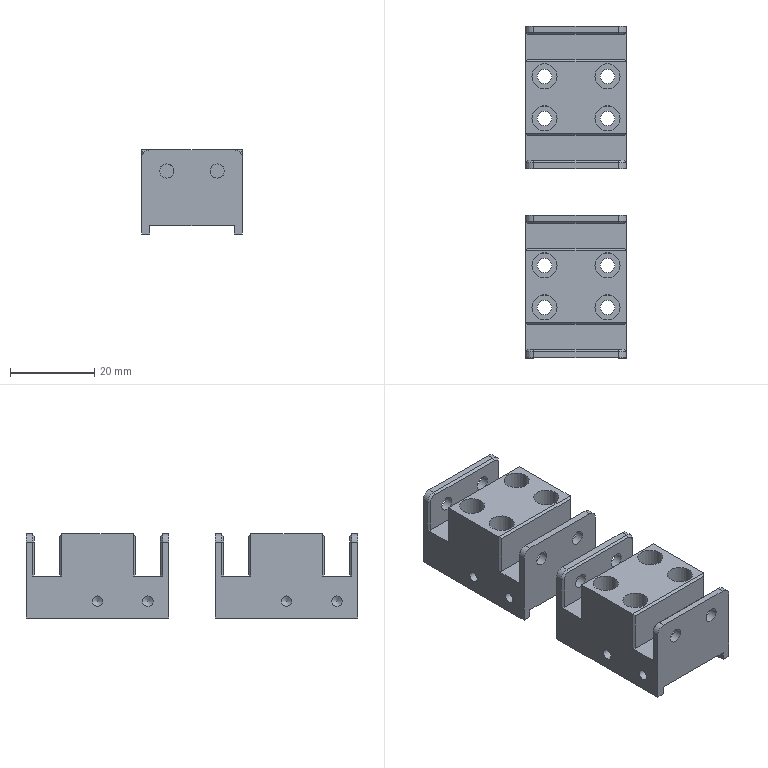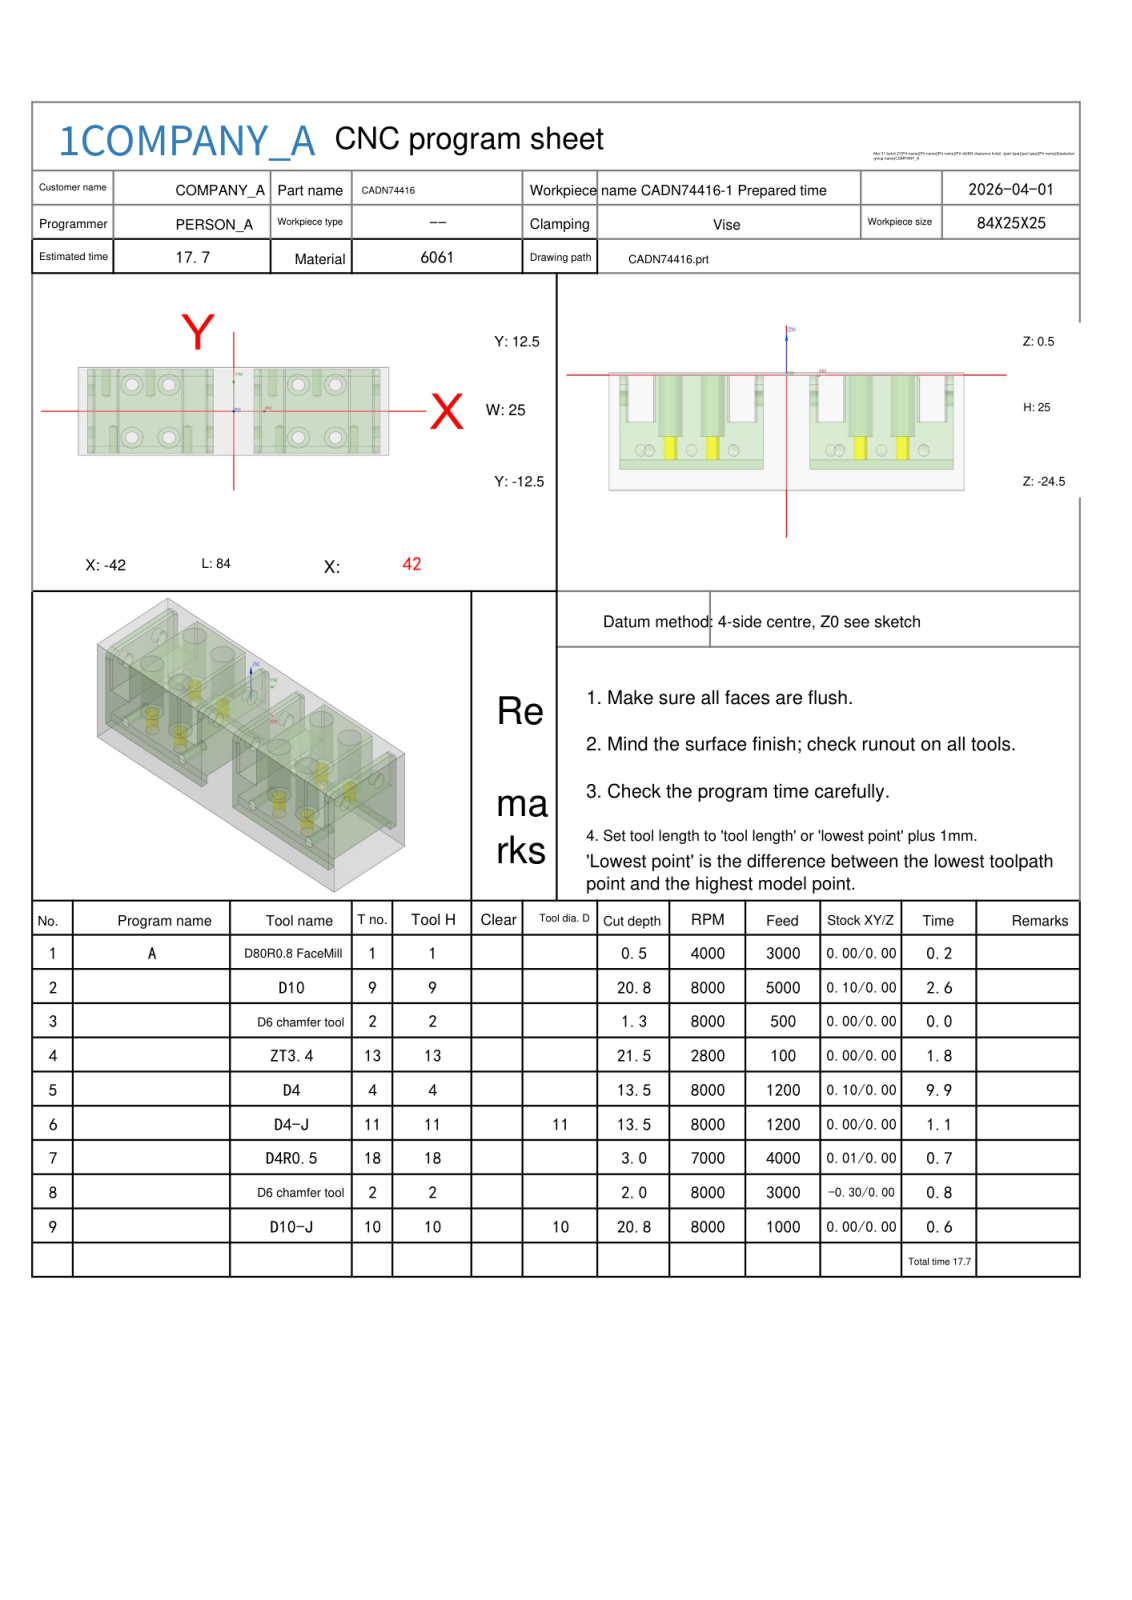NC program | NX | posted by the shop | part box 24 x 79 x 20 mm
Lines 4217 to 5292 of 7697:
N7 T18 M06
(D4R0.5  D=4. R=0.5 H=18 ce=0.01 di=0.00)
G00 G90 G54 X35.996 Y8.516 M03 S7000
G43 H18 Z10.5
M08
Z.491
G01 Z-.009 F4000.
X36.009 Y8.515
X36.024
G03 X36.424 Y8.9 I0.0 J.4
G01 X36.486 Y10.574
G02 X38. Y11.721 I1.656 J-.613
G01 X39.5
G03 X40.317 Y11.595 I.817 J2.584
X40.601 Y11.61 I0.0 J2.71
G01 Y11.646 Z-.014
Y11.681 Z-.018
G02 X39.5 Y11.812 I.04 J5.024
G01 X38.
G03 X36.378 Y10.29 I.095 J-1.726
G01 X36.373 Y10.255
X36.36 Y8.9
X36.326 Z-.03
X36.347 Y10.202
G02 X38. Y11.894 I1.721 J-.028
G01 X39.5
G03 X40.598 Y11.747 I1.098 J4.039
G01 X40.6
Y11.8 Z-.037
Y11.819 Z-.044
X39.5 Y11.976
X38.
G03 X36.315 Y10.23 I.098 J-1.781
G01 X36.288 Y8.9
X36.254 Z-.06
X36.278 Y10.29
X36.324 Y10.574
G02 X38. Y12.056 I1.748 J-.288
G01 X39.5
G02 X40.6 Y11.903 I-6.094 J-47.836
G01 Y11.957 Z-.07
Y11.997 Z-.08
G02 X39.5 Y12.136 I.262 J6.5
G01 X38.
G03 X36.302 Y10.663 I.069 J-1.795
G01 X36.234 Y10.29
X36.222 Y8.9
X36.188 Z-.102
X36.207 Y10.29
G02 X37.223 Y12.018 I2.097 J-.07
X38. Y12.217 I.939 J-2.054
G01 X39.5
G03 X40.6 Y12.068 I1.488 J6.815
G01 Y12.115 Z-.115
Y12.148 Z-.128
G02 X39.5 Y12.299 I.76 J9.617
G01 X38.
G03 X36.209 Y10.574 I.11 J-1.906
G01 X36.178 Y10.29
X36.158 Y8.9
X36.127 Y8.894 Z-.155
X36.146 Y10.29
G02 X36.881 Y11.951 I2.335 J-.04
X37.958 Y12.378 I1.077 J-1.145
G01 X39.5
G03 X40.6 Y12.235 I1.607 J8.064
G01 Y12.283 Z-.171
Y12.331 Z-.187
X39.5 Y12.458
X37.984
G03 X36.761 Y11.925 I0.0 J-1.67
X36.146 Y10.574 I1.718 J-1.597
G01 X36.111 Y10.29
X36.096 Y8.9
X36.06 Y8.894 Z-.223
X36.072 Y10.29
X36.089 Y10.434
G02 X36.373 Y11.477 I3.122 J-.289
X38. Y12.542 I1.687 J-.802
G01 X39.5
G03 X40.6 Y12.434 I1.179 J6.383
G01 Y12.478 Z-.243
Y12.518 Z-.263
G02 X39.5 Y12.626 I.066 J6.368
G01 X38.
G03 X36.373 Y11.579 I.04 J-1.851
X36.033 Y10.29 I3.27 J-1.551
X36.01 Y9.451 I15.233 J-.839
X36.02 Y8.896 I15.256 J0.0
G01 X35.977 Y8.898 Z-.306
G02 X35.966 Y9.452 I14.507 J.554
X35.985 Y10.182 I14.517 J0.0
X36.382 Y11.707 I3.875 J-.195
X38. Y12.709 I1.671 J-.893
G01 X39.5
G03 X40.579 Y12.604 I1.079 J5.501
G01 X40.6
Y12.648 Z-.33
Y12.692 Z-.353
X40.587
G02 X39.5 Y12.791 I0.0 J6.001
G01 X38.
G03 X36.373 Y11.786 I.054 J-1.906
X35.93 Y10.007 I3.595 J-1.84
G01 Y8.9
X35.879 Y8.902 Z-.404
Y10.007
G02 X36.29 Y11.707 I3.969 J-.06
G01 X36.373 Y11.883
G02 X38. Y12.873 I1.668 J-.91
G01 X39.5
G03 X40.6 Y12.787 I1.1 J7.015
G01 Y12.833 Z-.431
Y12.873 Z-.458
X40.469 Y12.872
G02 X39.5 Y12.953 I0.0 J5.854
G01 X38.
G03 X36.363 Y11.97 I.051 J-1.939
X35.833 Y10.171 I3.595 J-2.037
X35.812 Y9.456 I12.379 J-.716
X35.825 Y8.905 I12.4 J0.0
G01 X35.767 Y8.907 Z-.516
G02 X35.756 Y9.41 I11.375 J.503
X35.816 Y10.574 I11.386 J0.0
X36.373 Y12.071 I4.631 J-.871
X38. Y13.031 I1.67 J-.973
G01 X39.5
G03 X40.464 Y12.945 I.964 J5.378
G01 X40.6 Y12.947
Y12.992 Z-.546
Y13.024 Z-.577
X40.511
G02 X39.5 Y13.107 I0.0 J6.185
G01 X38.
G03 X36.507 Y12.346 I0.0 J-1.844
X35.709 Y10.007 I3.396 J-2.465
G01 X35.708 Y9.723
X35.706 Y8.911
X35.642 Y8.915 Z-.64
G02 X35.635 Y9.344 I11.989 J.429
X35.698 Y10.574 I11.996 J0.0
X36.388 Y12.274 I4.691 J-.913
X38. Y13.181 I1.646 J-1.039
G01 X39.5
X39.978 Y13.125
X40.058 Y13.109
X40.6 Y13.106
Y13.148 Z-.674
Y13.185 Z-.707
X40.492 Y13.184
G02 X39.5 Y13.253 I0.0 J7.2
G01 X38.
G03 X36.539 Y12.558 I.027 J-1.94
X35.635 Y10.574 I3.72 J-2.892
X35.57 Y9.33 I11.781 J-1.244
X35.576 Y8.925 I11.846 J0.0
G01 X35.542 Y8.927 Z-.742
X35.507 Y8.928 Z-.777
G02 X35.501 Y9.325 I11.376 J.397
X35.569 Y10.574 I11.383 J0.0
X36.574 Y12.666 I4.608 J-.927
X37.981 Y13.322 I1.406 J-1.178
G01 X39.5
G03 X40.43 Y13.263 I.93 J7.353
G01 X40.6 Y13.265
Y13.294 Z-.813
Y13.324 Z-.848
X40.058
X39.5 Y13.387
X37.983
G03 X36.575 Y12.737 I0.0 J-1.852
X35.503 Y10.574 I3.756 J-3.208
X35.431 Y9.297 I11.257 J-1.277
X35.437 Y8.932 I11.329 J0.0
G01 X35.401 Y8.933 Z-.883
X35.367 Y8.935 Z-.919
X35.379 Y9.894
G02 X35.855 Y11.735 I4.011 J-.054
X36.504 Y12.728 I6.009 J-3.221
X38. Y13.446 I1.506 J-1.218
G01 X39.5
G02 X40.058 Y13.383 I-.204 J-4.246
G01 X40.6 Y13.382
Y13.412 Z-.954
Y13.44 Z-.99
X40.058
X39.5 Y13.502
X38.
G03 X36.478 Y12.751 I.012 J-1.94
G01 X36.373 Y12.613
G03 X35.375 Y10.574 I3.809 J-3.128
X35.292 Y9.232 I10.9 J-1.342
X35.296 Y8.938 I10.983 J0.0
G01 X35.26 Y8.941 Z-1.025
X35.226 Y8.944 Z-1.06
G02 X35.222 Y9.212 I10.59 J.269
X35.31 Y10.574 I10.593 J0.0
X35.891 Y11.991 I4.369 J-.963
X36.452 Y12.774 I5.899 J-3.636
G01 X36.499 Y12.841
G02 X38. Y13.554 I1.518 J-1.259
G01 X39.5
X40.058 Y13.497
X40.6
Y13.524 Z-1.096
Y13.553 Z-1.131
G02 X40.399 Y13.55 I-.201 J7.883
X39.5 Y13.602 I0.0 J7.886
G01 X38.
G03 X36.457 Y12.841 I.017 J-1.98
G01 X36.426 Y12.797
G03 X35.806 Y11.939 I6.249 J-5.176
X35.246 Y10.574 I3.813 J-2.361
X35.152 Y9.23 I9.557 J-1.344
X35.156 Y8.961 I9.651 J0.0
G01 X35.119 Y8.969 Z-1.166
X35.085 Y8.977 Z-1.202
X35.104 Y9.898
G02 X35.481 Y11.431 I3.613 J-.074
X36.373 Y12.783 I5.933 J-2.945
G01 X36.401 Y12.82
G02 X38. Y13.646 I1.623 J-1.179
G01 X39.5
G03 X40.403 Y13.589 I.903 J7.075
G01 X40.6 Y13.592
Y13.614 Z-1.237
Y13.631 Z-1.272
X40.058
X39.5 Y13.688
X37.999
G03 X36.566 Y13.059 I0.0 J-1.946
X35.424 Y11.436 I5.641 J-5.183
X35.034 Y9.931 I3.02 J-1.585
G01 X35.016 Y9.156
X35.015 Y8.994
X34.946 Y9.104 Z-1.343
X34.963 Y9.924
G02 X35.422 Y11.531 I3.288 J-.069
G01 X35.526 Y11.707
G02 X36.492 Y13.016 I6.445 J-3.746
G01 X36.515 Y13.043
G02 X37.995 Y13.726 I1.48 J-1.262
G01 X39.5
G02 X40.058 Y13.67 I-.527 J-7.984
G01 X40.6
Y13.689 Z-1.378
Y13.708 Z-1.414
G02 X40.398 Y13.705 I-.202 J7.153
X39.5 Y13.762 I0.0 J7.156
G01 X38.
G03 X36.551 Y13.125 I.019 J-2.012
G01 X36.475 Y13.033
G03 X35.473 Y11.707 I5.965 J-5.548
G01 X35.381 Y11.557
G03 X34.882 Y9.796 I2.864 J-1.761
G01 X34.885 Y9.655
X34.874 Y9.773 Z-1.426
X34.864 Y9.892 Z-1.438
X34.855 Y10.011 Z-1.449
X34.853 Y10.13 Z-1.461
X34.856 Y10.248 Z-1.473
X34.865 Y10.364 Z-1.485
G02 X35.297 Y11.515 I2.945 J-.449
G01 X35.419 Y11.707
G02 X36.457 Y13.05 I7.546 J-4.759
G01 X36.516 Y13.125
G02 X38. Y13.795 I1.506 J-1.357
G01 X39.5
G03 X40.38 Y13.743 I.88 J7.429
X40.6 Y13.746 I0.0 J7.481
G01 Y13.766 Z-1.523
Y13.779 Z-1.56
G02 X40.349 Y13.775 I-.251 J6.979
X39.5 Y13.826 I0.0 J6.984
G01 X38.
G03 X36.486 Y13.125 I.019 J-2.025
G01 X36.438 Y13.067
G03 X35.222 Y11.485 I7.736 J-7.209
X34.932 Y10.908 I2.855 J-1.795
G01 X34.948 Y11.013 Z-1.586
X34.972 Y11.116 Z-1.613
X35.001 Y11.216 Z-1.639
G02 X35.303 Y11.707 I3.689 J-1.926
G01 X35.522 Y12.003
G02 X36.577 Y13.253 I10.046 J-7.402
X37.997 Y13.857 I1.42 J-1.366
G01 X39.5
X40.058 Y13.808
X40.6 Y13.809
Y13.826 Z-1.681
Y13.841 Z-1.723
G02 X40.363 Y13.837 I-.237 J7.591
X39.5 Y13.886 I0.0 J7.594
G01 X37.995
G03 X36.584 Y13.287 I0.0 J-1.96
G01 X36.428 Y13.125
G03 X35.695 Y12.274 I5.704 J-5.656
X35.066 Y11.449 I5.639 J-4.952
G01 X35.085 Y11.533 Z-1.767
X35.116 Y11.61 Z-1.811
G02 X35.653 Y12.274 I5.648 J-4.014
X36.373 Y13.094 I6.817 J-5.256
X38. Y13.913 I1.659 J-1.27
G01 X39.5
G03 X40.34 Y13.867 I.84 J7.621
X40.6 Y13.871 I0.0 J7.667
G01 Y13.888 Z-1.856
X40.599 Y13.903 Z-1.902
G02 X40.307 Y13.898 I-.293 J8.21
X39.5 Y13.937 I0.0 J8.215
G01 X37.995
G03 X36.577 Y13.336 I0.0 J-1.973
X35.157 Y11.747 I19.463 J-18.816
G01 X35.191 Y11.842 Z-1.995
G02 X36.623 Y13.408 I24.419 J-20.89
X38. Y13.958 I1.388 J-1.475
G01 X39.5
G03 X40.324 Y13.922 I.824 J9.323
X40.6 Y13.926 I0.0 J9.359
G01 Y13.939 Z-2.042
Y13.949 Z-2.09
G02 X40.289 Y13.945 I-.311 J9.859
X39.5 Y13.976 I0.0 J9.864
G01 X38.
G03 X36.603 Y13.408 I.008 J-2.022
G01 X36.048 Y12.841
G02 X35.227 Y11.938 I-22.757 J19.853
G01 X35.247 Y12. Z-2.187
G02 X36.587 Y13.408 I69.646 J-64.932
X38. Y13.99 I1.425 J-1.454
G01 X39.5
G03 X40.244 Y13.968 I.744 J12.471
X40.6 Y13.973 I0.0 J12.493
G01 X40.599 Y13.981 Z-2.226
X40.598 Y13.984 Z-2.265
G02 X40.257 Y13.98 I-.341 J15.166
X39.5 Y13.999 I0.0 J15.17
G01 X38.
X37.852 Y13.988
G03 X36.556 Y13.386 I.141 J-1.998
G01 X36.373 Y13.197
X35.248 Y12.023
X35.25 Y12.047 Z-2.343
X36.571 Y13.408
G02 X38. Y14.005 I1.446 J-1.452
G01 X39.5
G03 X40.261 Y13.991 I.761 J19.912
X40.598 Y13.993 I0.0 J19.927
G01 Y14.003 Z-2.422
X39.5 Y14.009
X37.996
G03 X36.57 Y13.41 I0.0 J-1.996
G01 X35.255 Y12.067
X35.259 Y12.088 Z-2.5
X35.44 Y12.274
X36.59 Y13.428
G02 X37.99 Y14.01 I1.4 J-1.395
G01 X40.598
G00 Z10.5
X41.016 Y-11.933
Z.491
G01 Z-.009
G03 X40.617 Y-11.56 I-.399 J-.027
G01 X40.601
G03 X39.5 Y-11.721 I.208 J-5.273
G01 X38.
G02 X36.486 Y-10.574 I.143 J1.76
G01 X36.424 Y-8.9
X36.384 Z-.014
X36.36 Z-.018
X36.362 Y-8.951
Y-10.083
G03 X38. Y-11.812 I1.731 J0.0
G01 X39.5
G02 X40.469 Y-11.691 I.969 J-3.817
G01 X40.6 Y-11.693
Y-11.748 Z-.024
Y-11.763 Z-.03
X40.428 Y-11.759
G03 X39.5 Y-11.894 I0.0 J-3.256
G01 X38.
G02 X36.347 Y-10.202 I.068 J1.72
G01 X36.325 Y-8.901
X36.288 Y-8.9 Z-.044
X36.316 Y-10.29
G03 X38. Y-11.976 I1.781 J.096
G01 X39.5
G02 X40.483 Y-11.838 I.983 J-3.45
G01 X40.6 Y-11.84
Y-11.9 Z-.052
Y-11.931 Z-.06
X40.538 Y-11.93
G03 X39.5 Y-12.056 I0.0 J-4.356
G01 X38.
G02 X36.324 Y-10.574 I.072 J1.77
G01 X36.278 Y-10.29
X36.255 Y-8.9
X36.222 Z-.08
X36.234 Y-10.29
X36.302 Y-10.663
G03 X38. Y-12.136 I1.767 J.322
G01 X39.5
G02 X40.475 Y-12.014 I.975 J-3.835
G01 X40.6 Y-12.016
Y-12.059 Z-.091
Y-12.084 Z-.102
X40.55
G03 X39.5 Y-12.217 I0.0 J-4.199
G01 X38.
G02 X36.424 Y-11.148 I.066 J1.793
X36.197 Y-10.085 I2.448 J1.079
G01 X36.19 Y-9.054
X36.188 Y-8.9
X36.158 Z-.128
X36.178 Y-10.29
X36.209 Y-10.574
G03 X38. Y-12.299 I1.901 J.181
G01 X39.5
G02 X40.6 Y-12.162 I1.306 J-6.004
G01 Y-12.209 Z-.142
Y-12.246 Z-.155
G03 X39.5 Y-12.378 I.197 J-6.301
G01 X38.
G02 X36.373 Y-11.257 I.048 J1.811
X36.133 Y-10.062 I2.862 J1.195
G01 X36.134 Y-10.007
X36.127 Y-8.894
X36.096 Y-8.899 Z-.187
X36.097 Y-10.007
Y-10.012
G03 X36.373 Y-11.368 I3.476 J0.0
X38. Y-12.458 I1.681 J.751
G01 X39.5
G02 X40.6 Y-12.337 I1.268 J-6.477
G01 Y-12.388 Z-.205
Y-12.434 Z-.223
G03 X39.5 Y-12.542 I.087 J-6.575
G01 X38.
G02 X36.349 Y-11.424 I.06 J1.866
X36.06 Y-10.012 I3.305 J1.412
G01 Y-10.007
Y-8.894
X36.02 Y-8.895 Z-.263
Y-10.007
G03 X36.373 Y-11.579 I3.716 J.007
X38. Y-12.626 I1.667 J.805
G01 X39.5
G02 X40.6 Y-12.518 I1.163 J-6.232
G01 Y-12.563 Z-.284
Y-12.604 Z-.306
X40.566
G03 X39.5 Y-12.709 I0.0 J-5.467
G01 X38.
G02 X36.373 Y-11.691 I.055 J1.897
X35.977 Y-10.007 I3.568 J1.728
G01 Y-8.897
X35.93 Y-8.899 Z-.353
Y-10.007
G03 X36.373 Y-11.786 I4.038 J.061
X38. Y-12.791 I1.681 J.901
G01 X39.5
G02 X40.56 Y-12.692 I1.06 J-5.606
G01 X40.6
Y-12.74 Z-.379
Y-12.787 Z-.404
X40.598
G03 X39.5 Y-12.873 I0.0 J-7.073
G01 X38.
G02 X36.373 Y-11.883 I.041 J1.9
G01 X36.29 Y-11.707
G02 X35.879 Y-10.007 I3.558 J1.76
G01 Y-8.901
X35.825 Y-8.903 Z-.458
Y-9.927
G03 X36.363 Y-11.97 I4.143 J0.0
X38. Y-12.953 I1.687 J.956
G01 X39.5
G02 X40.469 Y-12.872 I.969 J-5.773
G01 X40.6 Y-12.873
Y-12.917 Z-.487
Y-12.947 Z-.516
X40.472 Y-12.945
G03 X39.5 Y-13.031 I0.0 J-5.565
G01 X38.
G02 X36.507 Y-12.274 I.046 J1.943
X35.768 Y-10.007 I3.496 J2.394
G01 Y-9.723
X35.767 Y-8.906
X35.706 Y-8.911 Z-.577
X35.708 Y-9.877
G03 X36.502 Y-12.338 I4.23 J.005
X38. Y-13.107 I1.498 J1.076
G01 X39.5
G02 X40.511 Y-13.024 I1.011 J-6.102
G01 X40.6
Y-13.068 Z-.609
Y-13.106 Z-.64
X40.058 Y-13.109
X39.971 Y-13.125
X39.5 Y-13.181
X38.
G02 X36.61 Y-12.558 I.027 J1.922
X35.647 Y-10.007 I3.31 J2.707
G01 X35.644 Y-9.723
Y-8.934
X35.642 Y-8.915
X35.611 Y-8.919 Z-.674
X35.577 Y-8.924 Z-.707
G03 X35.57 Y-9.339 I11.758 J-.415
X35.635 Y-10.574 I11.765 J0.0
X36.539 Y-12.558 I4.623 J.908
X38. Y-13.253 I1.488 J1.245
G01 X39.5
G02 X40.492 Y-13.184 I.992 J-7.131
G01 X40.6 Y-13.185
Y-13.224 Z-.742
Y-13.265 Z-.777
G03 X40.395 Y-13.262 I-.205 J-6.74
X39.5 Y-13.322 I0.0 J-6.743
G01 X37.981
G02 X36.574 Y-12.665 I0.0 J1.835
X35.569 Y-10.574 I3.602 J3.018
X35.501 Y-9.339 I11.149 J1.235
X35.509 Y-8.928 I11.217 J0.0
G01 X35.473 Y-8.929 Z-.813
X35.438 Y-8.931 Z-.848
G03 X35.432 Y-9.31 I11.176 J-.379
X35.503 Y-10.574 I11.183 J0.0
X36.565 Y-12.727 I4.852 J1.053
X37.987 Y-13.387 I1.422 J1.203
G01 X39.5
X40.058 Y-13.324
X40.6
Y-13.354 Z-.883
Y-13.382 Z-.919
X40.058 Y-13.383
G02 X39.5 Y-13.446 I-.762 J4.182
G01 X38.
G02 X36.504 Y-12.728 I.01 J1.937
X36.089 Y-12.134 I4.293 J3.441
G01 X35.999 Y-11.991
G02 X35.375 Y-9.86 I3.436 J2.163
G01 X35.368 Y-8.934
X35.332 Y-8.936 Z-.954
X35.298 Y-8.938 Z-.99
G03 X35.293 Y-9.26 I10.543 J-.322
X35.375 Y-10.574 I10.548 J0.0
X36.329 Y-12.558 I4.786 J1.079
G01 X36.373 Y-12.613
X36.478 Y-12.751
G03 X38. Y-13.502 I1.533 J1.189
G01 X39.5
X39.774 Y-13.479
X40.058 Y-13.44
X40.6
Y-13.47 Z-1.025
Y-13.497 Z-1.06
X40.058
X39.774 Y-13.533
X39.5 Y-13.554
X38.
G02 X36.452 Y-12.774 I.006 J1.938
G01 X36.197 Y-12.44
G02 X35.504 Y-11.225 I4.165 J3.182
X35.245 Y-9.97 I3.295 J1.334
G01 X35.227 Y-9.156
X35.228 Y-8.944
X35.158 Y-8.964 Z-1.131
X35.172 Y-9.909
G03 X35.476 Y-11.298 I3.588 J.057
X36.239 Y-12.558 I5.2 J2.287
G01 X36.373 Y-12.726
X36.426 Y-12.797
G03 X38. Y-13.602 I1.586 J1.16
G01 X39.5
G02 X40.368 Y-13.549 I.868 J-7.123
X40.6 Y-13.553 I0.0 J-7.175
G01 Y-13.572 Z-1.166
Y-13.592 Z-1.202
G03 X40.395 Y-13.589 I-.204 J-6.983
X39.5 Y-13.646 I0.0 J-6.986
G01 X38.
G02 X36.401 Y-12.82 I.024 J2.006
G01 X36.373 Y-12.783
X36.194 Y-12.558
G02 X35.438 Y-11.34 I4.461 J3.611
X35.104 Y-9.886 I3.345 J1.534
G01 X35.088 Y-9.156
Y-8.983
X35.018 Y-9.002 Z-1.272
Y-9.156
X35.035 Y-9.922
G03 X35.426 Y-11.439 I3.422 J.073
X36.566 Y-13.059 I6.761 J3.548
X37.999 Y-13.688 I1.433 J1.317
G01 X39.5
X39.774 Y-13.666
X40.058 Y-13.631
X40.6
Y-13.651 Z-1.308
Y-13.67 Z-1.343
X40.058
X39.867 Y-13.692
X39.5 Y-13.726
X38.
G02 X36.585 Y-13.125 I.015 J2.
G01 X36.215 Y-12.692
G02 X35.522 Y-11.7 I4.803 J4.096
G01 X35.424 Y-11.534
G02 X34.965 Y-9.926 I2.831 J1.677
G01 X34.949 Y-9.156
Y-9.092
X34.933 Y-9.227 Z-1.361
X34.919 Y-9.362 Z-1.378
X34.904 Y-9.496 Z-1.396
X34.891 Y-9.631 Z-1.414
X34.887 Y-9.806
G03 X35.381 Y-11.557 I3.349 J0.0
G01 X35.473 Y-11.707
G03 X36.229 Y-12.751 I6.196 J3.691
G01 X36.475 Y-13.033
X36.551 Y-13.125
G03 X38. Y-13.762 I1.466 J1.368
G01 X39.5
G02 X40.385 Y-13.705 I.885 J-6.826
X40.6 Y-13.708 I0.0 J-6.884
G01 Y-13.727 Z-1.449
Y-13.746 Z-1.485
G03 X40.351 Y-13.742 I-.249 J-6.829
X39.5 Y-13.795 I0.0 J-6.834
G01 X38.
G02 X36.516 Y-13.125 I.02 J2.021
G01 X36.457 Y-13.05
G02 X35.419 Y-11.707 I6.501 J6.095
G01 X35.294 Y-11.511
G02 X34.866 Y-10.35 I2.488 J1.579
G01 Y-10.492 Z-1.504
X34.881 Y-10.631 Z-1.523
X34.902 Y-10.769 Z-1.541
X34.931 Y-10.904 Z-1.56
G03 X35.211 Y-11.468 I3.121 J1.198
X36.237 Y-12.841 I8.47 J5.256
G01 X36.438 Y-13.067
X36.486 Y-13.125
G03 X38. Y-13.826 I1.531 J1.319
G01 X39.5
G02 X40.363 Y-13.775 I.863 J-7.159
X40.6 Y-13.779 I0.0 J-7.211
G01 Y-13.798 Z-1.6
Y-13.808 Z-1.639
X40.058
X39.5 Y-13.857
X37.998
G02 X36.582 Y-13.256 I0.0 J1.969
G01 X36.455 Y-13.125
G02 X35.522 Y-12.003 I9.198 J8.598
G01 X35.303 Y-11.707
G02 X35.001 Y-11.213 I3.469 J2.46
G01 X35.026 Y-11.334 Z-1.681
X35.065 Y-11.446 Z-1.723
G03 X35.695 Y-12.274 I5.88 J3.816
X36.428 Y-13.125 I6.451 J4.818
G01 X36.585 Y-13.288
G03 X37.994 Y-13.886 I1.409 J1.36
G01 X39.5
G02 X40.42 Y-13.836 I.92 J-8.384
G01 X40.6 Y-13.838
Y-13.852 Z-1.767
Y-13.867 Z-1.811
X40.442 Y-13.865
G03 X39.5 Y-13.913 I0.0 J-9.247
G01 X37.989
G02 X36.581 Y-13.312 I0.0 J1.948
G01 X36.204 Y-12.917
G02 X35.653 Y-12.274 I5.524 J5.283
X35.117 Y-11.608 I4.596 J4.251
G01 X35.132 Y-11.681 Z-1.856
X35.156 Y-11.747 Z-1.902
G03 X36.575 Y-13.334 I21.32 J17.633
X37.996 Y-13.937 I1.421 J1.372
G01 X39.5
G02 X40.446 Y-13.895 I.946 J-10.506
G01 X40.6 Y-13.896
Y-13.908 Z-1.948
Y-13.921 Z-1.995
X40.434 Y-13.919
G03 X39.5 Y-13.958 I0.0 J-11.19
G01 X38.
G02 X36.623 Y-13.408 I.011 J2.026
X35.19 Y-11.842 I23.469 J22.914
G01 X35.226 Y-11.937 Z-2.09
G02 X36.048 Y-12.841 I-17.148 J-16.428
G01 X36.603 Y-13.408
G03 X38. Y-13.976 I1.405 J1.453
G01 X39.5
G02 X40.483 Y-13.943 I.983 J-14.629
G01 X40.6 Y-13.944
Y-13.958 Z-2.138
Y-13.967 Z-2.187
X40.582
G03 X39.5 Y-13.99 I0.0 J-25.192
G01 X38.
G02 X36.656 Y-13.474 I.014 J2.042
X35.782 Y-12.558 I11.132 J11.5
G01 X35.245 Y-12.001
X35.246 Y-12.025 Z-2.265
X35.806 Y-12.598
G03 X36.692 Y-13.514 I12.701 J11.398
X38. Y-13.999 I1.35 J1.638
G01 X39.5
G02 X40.385 Y-13.98 I.885 J-21.05
X40.598 Y-13.981 I0.0 J-21.069
G01 Y-13.983 Z-2.304
Y-13.992 Z-2.343
G03 X40.362 Y-13.991 I-.236 J-25.915
X39.5 Y-14.005 I0.0 J-25.916
G01 X38.
G02 X36.571 Y-13.408 I.018 J2.052
G03 X35.248 Y-12.048 I-257.754 J-249.448
G01 X35.254 Y-12.068 Z-2.422
X36.567 Y-13.408
G03 X38. Y-14.009 I1.439 J1.423
G01 X39.5
X40.598 Y-14.002
Y-14.01 Z-2.5
X37.967
G02 X36.607 Y-13.449 I.033 J2.009
G01 X35.259 Y-12.088
G00 Z10.5
X-4.153 Y-11.956
Z.491
G01 Z-.009
X-4.178 Y-11.734
G03 X-4.377 Y-11.557 I-.199 J-.022
G01 X-4.4 Y-11.558
G03 X-5.5 Y-11.721 I1.785 J-15.854
G01 X-7.
G02 X-8.542 Y-10.29 I.036 J1.585
G01 X-8.574 Y-8.9
X-8.642 Z-.018
X-8.64 Y-8.955
Y-10.007
X-8.635 Y-10.148
G03 X-7. Y-11.812 I1.728 J.062
G01 X-5.5
G02 X-4.537 Y-11.692 I.962 J-3.778
G01 X-4.4 Y-11.694
Y-11.748 Z-.024
Y-11.764 Z-.03
X-4.577 Y-11.759
G03 X-5.5 Y-11.894 I0.0 J-3.226
G01 X-7.
G02 X-8.654 Y-10.2 I.069 J1.722
G01 X-8.676 Y-8.901
X-8.712 Y-8.9 Z-.044
X-8.684 Y-10.29
G03 X-7. Y-11.976 I1.781 J.096
G01 X-5.5
G02 X-4.525 Y-11.839 I.975 J-3.407
G01 X-4.4 Y-11.841
Y-11.9 Z-.052
Y-11.932 Z-.06
X-4.474 Y-11.931
G03 X-5.5 Y-12.056 I0.0 J-4.276
G01 X-7.
G02 X-8.676 Y-10.574 I.075 J1.774
G01 X-8.721 Y-10.29
X-8.745 Y-8.9
X-8.777 Z-.08
X-8.764 Y-10.29
X-8.699 Y-10.657
G03 X-7. Y-12.136 I1.766 J.313
G01 X-5.5
G02 X-4.533 Y-12.014 I.967 J-3.785
G01 X-4.4 Y-12.016
Y-12.059 Z-.091
Y-12.085 Z-.102
X-4.457 Y-12.084
G03 X-5.5 Y-12.217 I0.0 J-4.156
G01 X-7.
G02 X-8.579 Y-11.14 I.065 J1.791
X-8.805 Y-10.062 I2.456 J1.078
G01 Y-10.007
Y-9.048
X-8.812 Y-8.9
X-8.842 Z-.128
X-8.823 Y-10.29
X-8.792 Y-10.574
G03 X-7. Y-12.299 I1.915 J.195
G01 X-5.5
G02 X-4.4 Y-12.163 I1.29 J-5.894
G01 Y-12.209 Z-.142
Y-12.246 Z-.155
G03 X-5.5 Y-12.378 I.222 J-6.525
G01 X-7.
G02 X-8.632 Y-11.247 I.048 J1.812
X-8.867 Y-10.063 I2.87 J1.184
G01 X-8.866 Y-10.007
Y-9.082
X-8.873 Y-8.893
X-8.904 Y-8.898 Z-.187
X-8.902 Y-10.007
Y-10.019
G03 X-8.632 Y-11.357 I3.452 J0.0
X-7. Y-12.458 I1.687 J.74
G01 X-5.5
G02 X-4.4 Y-12.337 I1.276 J-6.566
G01 Y-12.388 Z-.205
Y-12.434 Z-.223
G03 X-5.5 Y-12.542 I.127 J-6.994
G01 X-7.
G02 X-8.652 Y-11.424 I.06 J1.868
X-8.94 Y-10.008 I3.333 J1.415
G01 Y-10.007
Y-8.894
X-8.98 Y-8.896 Z-.263
Y-10.007
G03 X-8.632 Y-11.57 I3.718 J.007
X-7. Y-12.626 I1.673 J.797
G01 X-5.5
G02 X-4.4 Y-12.518 I1.175 J-6.358
G01 Y-12.563 Z-.284
Y-12.604 Z-.306
X-4.408
G03 X-5.5 Y-12.709 I0.0 J-5.746
G01 X-7.
G02 X-8.648 Y-11.649 I.054 J1.896
X-9.023 Y-10.035 I3.287 J1.615
G01 Y-8.897
X-9.07 Y-8.899 Z-.353
Y-10.007
G03 X-8.632 Y-11.777 I4.05 J.063
X-7. Y-12.791 I1.686 J.894
G01 X-5.5
G02 X-4.421 Y-12.692 I1.079 J-5.824
G01 X-4.4
Y-12.74 Z-.379
Y-12.787 Z-.404
G03 X-5.5 Y-12.873 I.017 J-7.331
G01 X-7.
G02 X-8.632 Y-11.874 I.042 J1.902
G01 X-8.711 Y-11.707
G02 X-9.121 Y-10.007 I3.576 J1.763
G01 Y-8.901
X-9.175 Y-8.903 Z-.458
Y-9.95
G03 X-8.802 Y-11.617 I3.909 J0.0
G01 X-8.632 Y-11.977
G03 X-7. Y-12.953 I1.682 J.961
G01 X-5.5
G02 X-4.523 Y-12.872 I.977 J-5.89
G01 X-4.4 Y-12.873
Y-12.917 Z-.487
Y-12.947 Z-.516
X-4.529 Y-12.945
G03 X-5.5 Y-13.031 I0.0 J-5.562
G01 X-7.
G02 X-8.494 Y-12.274 I.047 J1.945
X-9.232 Y-10.007 I3.503 J2.395
G01 X-9.233 Y-9.723
Y-8.906
X-9.294 Y-8.911 Z-.577
X-9.293 Y-9.723
X-9.292 Y-9.898
G03 X-8.497 Y-12.341 I4.221 J.022
X-7.003 Y-13.107 I1.494 J1.075
G01 X-5.5
G02 X-4.479 Y-13.024 I1.021 J-6.243
G01 X-4.4 Y-13.025
Y-13.068 Z-.609
Y-13.106 Z-.64
X-4.953 Y-13.111
X-5.027 Y-13.125
X-5.5 Y-13.181
X-7.
G02 X-8.39 Y-12.558 I.028 J1.924
X-9.353 Y-10.007 I3.315 J2.709
G01 X-9.356 Y-9.723
Y-8.935
X-9.358 Y-8.915
X-9.389 Y-8.919 Z-.674
X-9.423 Y-8.924 Z-.707
G03 X-9.43 Y-9.339 I11.755 J-.415
X-9.365 Y-10.574 I11.763 J0.0
X-8.461 Y-12.558 I4.612 J.904
X-7. Y-13.253 I1.487 J1.242
G01 X-5.5
G02 X-4.499 Y-13.184 I1.001 J-7.291
G01 X-4.4 Y-13.185
Y-13.224 Z-.742
Y-13.265 Z-.777
X-4.566 Y-13.263
G03 X-5.5 Y-13.322 I0.0 J-7.501
G01 X-7.019
G02 X-8.428 Y-12.663 I0.0 J1.837
X-9.431 Y-10.574 I3.605 J3.015
X-9.499 Y-9.339 I11.101 J1.234
X-9.491 Y-8.928 I11.169 J0.0
G01 X-9.527 Y-8.929 Z-.813
X-9.562 Y-8.931 Z-.848
G03 X-9.568 Y-9.311 I11.147 J-.38
X-9.496 Y-10.574 I11.154 J0.0
X-8.445 Y-12.714 I4.837 J1.046
X-7.001 Y-13.387 I1.445 J1.216
G01 X-5.5
X-4.953 Y-13.326
X-4.4 Y-13.324
Y-13.354 Z-.883
Y-13.382 Z-.919
X-4.953 Y-13.384
G02 X-5.5 Y-13.446 I-.732 J3.968
G01 X-7.
G02 X-8.499 Y-12.725 I.012 J1.943
X-9.133 Y-11.759 I5.611 J4.373
X-9.622 Y-9.885 I3.515 J1.917
G01 X-9.632 Y-8.934
X-9.668 Y-8.936 Z-.954
X-9.702 Y-8.938 Z-.99
G03 X-9.707 Y-9.26 I10.543 J-.322
X-9.625 Y-10.574 I10.548 J0.0
X-8.671 Y-12.558 I4.793 J1.083
G01 X-8.632 Y-12.607
X-8.524 Y-12.748
G03 X-7. Y-13.502 I1.537 J1.189
G01 X-5.5
X-4.953 Y-13.441
X-4.4 Y-13.44
Y-13.47 Z-1.025
Y-13.497 Z-1.06
X-4.953 Y-13.498
X-5.5 Y-13.554
X-7.
G02 X-8.632 Y-12.663 I.016 J1.969
X-9.689 Y-10.574 I3.766 J3.218
X-9.777 Y-9.237 I10.18 J1.336
X-9.772 Y-8.944 I10.267 J0.0
G01 X-9.842 Y-8.97 Z-1.131
X-9.827 Y-9.908
G03 X-9.523 Y-11.301 I3.599 J.058
X-8.761 Y-12.558 I5.189 J2.285
G01 X-8.632 Y-12.719
X-8.576 Y-12.793
G03 X-7. Y-13.602 I1.588 J1.156
G01 X-5.5
G02 X-4.632 Y-13.549 I.868 J-7.149
X-4.4 Y-13.553 I0.0 J-7.202
G01 Y-13.572 Z-1.166
Y-13.592 Z-1.202
X-4.953
X-5.236 Y-13.624
X-5.5 Y-13.646
X-7.
G02 X-8.602 Y-12.816 I.023 J2.003
G01 X-8.632 Y-12.776
X-8.806 Y-12.558
G02 X-9.581 Y-11.302 I4.61 J3.71
X-9.897 Y-9.903 I3.197 J1.457
G01 X-9.912 Y-8.995
X-9.982 Y-9.021 Z-1.272
Y-9.156
X-9.965 Y-9.922
G03 X-9.578 Y-11.43 I3.421 J.073
X-8.42 Y-13.071 I6.651 J3.467
X-7.004 Y-13.688 I1.417 J1.317
G01 X-5.5
G03 X-4.953 Y-13.631 I-.286 J5.423
G01 X-4.4
Y-13.651 Z-1.308
Y-13.67 Z-1.343
G03 X-4.67 Y-13.659 I-.27 J-3.292
X-5.136 Y-13.692 I0.0 J-3.303
G01 X-5.236 Y-13.706
X-5.5 Y-13.726
X-7.
G02 X-8.415 Y-13.125 I.013 J1.996
G01 X-8.733 Y-12.756
G02 X-9.481 Y-11.695 I5.053 J4.357
G01 X-9.578 Y-11.531
G02 X-10.035 Y-9.923 I2.83 J1.673
G01 X-10.051 Y-9.093
X-10.067 Y-9.227 Z-1.361
X-10.081 Y-9.362 Z-1.378
X-10.096 Y-9.496 Z-1.396
X-10.109 Y-9.631 Z-1.414
X-10.113 Y-9.805
G03 X-9.619 Y-11.557 I3.353 J0.0
G01 X-9.527 Y-11.707
G03 X-8.83 Y-12.679 I6.047 J3.6
G01 X-8.449 Y-13.125
G03 X-7. Y-13.762 I1.468 J1.374
G01 X-5.5
X-4.953 Y-13.708
X-4.4
Y-13.727 Z-1.449
Y-13.746 Z-1.485
G03 X-4.652 Y-13.741 I-.252 J-6.764
X-5.5 Y-13.795 I0.0 J-6.769
G01 X-7.
G02 X-8.483 Y-13.125 I.022 J2.026
G01 X-8.632 Y-12.949
X-8.728 Y-12.841
G02 X-9.581 Y-11.707 I6.278 J5.61
G01 X-9.706 Y-11.511
G02 X-10.135 Y-10.35 I2.487 J1.579
G01 X-10.134 Y-10.492 Z-1.504
X-10.119 Y-10.631 Z-1.523
X-10.098 Y-10.77 Z-1.541
X-10.069 Y-10.905 Z-1.56
G03 X-9.796 Y-11.463 I2.63 J.939
X-8.349 Y-13.294 I9.618 J6.112
X-7. Y-13.826 I1.371 J1.5
G01 X-5.5
G02 X-4.637 Y-13.775 I.863 J-7.176
X-4.4 Y-13.779 I0.0 J-7.228
G01 Y-13.798 Z-1.6
Y-13.808 Z-1.639
X-4.953 Y-13.809
X-5.5 Y-13.857
X-7.005
G02 X-8.421 Y-13.254 I0.0 J1.964
X-9.884 Y-11.424 I9.275 J8.915
G01 X-9.999 Y-11.213
X-9.974 Y-11.334 Z-1.681
X-9.935 Y-11.447 Z-1.723
G03 X-9.305 Y-12.274 I6.115 J4.001
X-8.379 Y-13.324 I7.645 J5.814
X-7.001 Y-13.886 I1.378 J1.408
G01 X-5.5
G02 X-4.582 Y-13.836 I.918 J-8.34
G01 X-4.4 Y-13.838
Y-13.852 Z-1.767
Y-13.867 Z-1.811
X-4.56 Y-13.865
G03 X-5.5 Y-13.913 I0.0 J-9.228
G01 X-7.007
G02 X-8.379 Y-13.352 I0.0 J1.956
X-9.347 Y-12.274 I8.151 J8.294
X-9.885 Y-11.609 I5.005 J4.597
G01 X-9.868 Y-11.682 Z-1.856
X-9.843 Y-11.748 Z-1.902
G03 X-8.427 Y-13.333 I21.597 J17.873
X-7.004 Y-13.937 I1.423 J1.372
G01 X-5.5
G02 X-4.559 Y-13.895 I.941 J-10.415
G01 X-4.4 Y-13.896
Y-13.908 Z-1.948
Y-13.921 Z-1.995
X-4.571 Y-13.919
G03 X-5.5 Y-13.958 I0.0 J-11.081
G01 X-7.
G02 X-8.378 Y-13.408 I.012 J2.03
X-9.808 Y-11.845 I24.159 J23.547
G01 X-9.771 Y-11.944 Z-2.09
G02 X-8.952 Y-12.841 I-15.236 J-14.739
G01 X-8.423 Y-13.379
G03 X-7. Y-13.976 I1.424 J1.398
G01 X-5.5
G02 X-4.528 Y-13.943 I.972 J-14.353
G01 X-4.4 Y-13.944
Y-13.958 Z-2.138
Y-13.967 Z-2.187
X-4.443
G03 X-5.5 Y-13.99 I0.0 J-24.242
G01 X-7.
G02 X-8.327 Y-13.489 I.014 J2.042
X-9.219 Y-12.558 I10.552 J11.003
G01 X-9.755 Y-12.001
X-9.754 Y-12.025 Z-2.265
G02 X-8.506 Y-13.325 I-183.211 J-177.098
G03 X-8.066 Y-13.692 I1.824 J1.738
X-7. Y-13.999 I1.113 J1.864
G01 X-5.5
G02 X-4.609 Y-13.98 I.891 J-21.221
X-4.396 Y-13.981 I0.0 J-21.239
G01 Y-13.983 Z-2.304
Y-13.992 Z-2.343